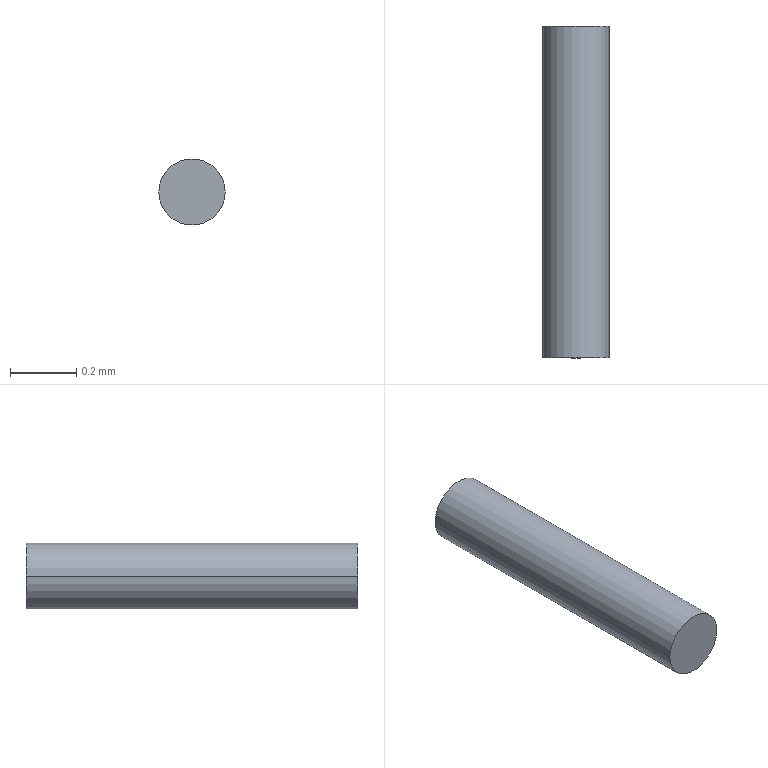Part | STEP file | Guide wheel mechanism revised.sldasm-Part-434 | 1 solid | 4 faces | box 0.2 x 1 x 0.2 mm | volume 0.03142 mm3 | cylinder 2 | plane 2 | commonest cylinder face diameters 0.2 x2
STEP:
#1=CARTESIAN_POINT('',(0.1,1.,0.));
#2=VERTEX_POINT('',#1);
#3=CARTESIAN_POINT('',(-0.1,1.,0.));
#4=VERTEX_POINT('',#3);
#5=CARTESIAN_POINT('',(0.,1.,0.));
#6=DIRECTION('',(0.,-1.,0.));
#7=DIRECTION('',(1.,0.,0.));
#8=AXIS2_PLACEMENT_3D('',#5,#6,#7);
#9=CIRCLE('',#8,0.1);
#10=EDGE_CURVE('',#2,#4,#9,.T.);
#11=ORIENTED_EDGE('',*,*,#10,.T.);
#12=CARTESIAN_POINT('',(-0.1,0.,0.));
#13=VERTEX_POINT('',#12);
#14=CARTESIAN_POINT('',(-0.1,1.,0.));
#15=DIRECTION('',(0.,-1.,0.));
#16=VECTOR('',#15,1000.);
#17=LINE('',#14,#16);
#18=EDGE_CURVE('',#4,#13,#17,.T.);
#19=ORIENTED_EDGE('',*,*,#18,.T.);
#20=CARTESIAN_POINT('',(0.1,0.,0.));
#21=VERTEX_POINT('',#20);
#22=CARTESIAN_POINT('',(0.,0.,0.));
#23=DIRECTION('',(0.,-1.,0.));
#24=DIRECTION('',(1.,0.,0.));
#25=AXIS2_PLACEMENT_3D('',#22,#23,#24);
#26=CIRCLE('',#25,0.1);
#27=EDGE_CURVE('',#21,#13,#26,.T.);
#28=ORIENTED_EDGE('',*,*,#27,.F.);
#29=CARTESIAN_POINT('',(0.1,1.,0.));
#30=DIRECTION('',(0.,-1.,0.));
#31=VECTOR('',#30,1000.);
#32=LINE('',#29,#31);
#33=EDGE_CURVE('',#2,#21,#32,.T.);
#34=ORIENTED_EDGE('',*,*,#33,.F.);
#35=EDGE_LOOP('',(#11,#19,#28,#34));
#36=FACE_OUTER_BOUND('',#35,.T.);
#37=CARTESIAN_POINT('',(0.,1.,0.));
#38=DIRECTION('',(0.,-1.,0.));
#39=DIRECTION('',(1.,0.,0.));
#40=AXIS2_PLACEMENT_3D('',#37,#38,#39);
#41=CYLINDRICAL_SURFACE('',#40,0.1);
#42=ADVANCED_FACE('',(#36),#41,.T.);
#43=ORIENTED_EDGE('',*,*,#18,.F.);
#44=CARTESIAN_POINT('',(0.,1.,0.));
#45=DIRECTION('',(0.,-1.,0.));
#46=DIRECTION('',(1.,0.,0.));
#47=AXIS2_PLACEMENT_3D('',#44,#45,#46);
#48=CIRCLE('',#47,0.1);
#49=EDGE_CURVE('',#4,#2,#48,.T.);
#50=ORIENTED_EDGE('',*,*,#49,.T.);
#51=ORIENTED_EDGE('',*,*,#33,.T.);
#52=CARTESIAN_POINT('',(0.,0.,0.));
#53=DIRECTION('',(0.,-1.,0.));
#54=DIRECTION('',(1.,0.,0.));
#55=AXIS2_PLACEMENT_3D('',#52,#53,#54);
#56=CIRCLE('',#55,0.1);
#57=EDGE_CURVE('',#13,#21,#56,.T.);
#58=ORIENTED_EDGE('',*,*,#57,.F.);
#59=EDGE_LOOP('',(#43,#50,#51,#58));
#60=FACE_OUTER_BOUND('',#59,.T.);
#61=CARTESIAN_POINT('',(0.,1.,0.));
#62=DIRECTION('',(0.,-1.,0.));
#63=DIRECTION('',(1.,0.,0.));
#64=AXIS2_PLACEMENT_3D('',#61,#62,#63);
#65=CYLINDRICAL_SURFACE('',#64,0.1);
#66=ADVANCED_FACE('',(#60),#65,.T.);
#67=ORIENTED_EDGE('',*,*,#10,.F.);
#68=ORIENTED_EDGE('',*,*,#49,.F.);
#69=EDGE_LOOP('',(#67,#68));
#70=FACE_OUTER_BOUND('',#69,.T.);
#71=CARTESIAN_POINT('',(0.,1.,0.));
#72=DIRECTION('',(0.,-1.,0.));
#73=DIRECTION('',(1.,0.,0.));
#74=AXIS2_PLACEMENT_3D('',#71,#72,#73);
#75=PLANE('',#74);
#76=ADVANCED_FACE('',(#70),#75,.F.);
#77=ORIENTED_EDGE('',*,*,#27,.T.);
#78=ORIENTED_EDGE('',*,*,#57,.T.);
#79=EDGE_LOOP('',(#77,#78));
#80=FACE_OUTER_BOUND('',#79,.T.);
#81=CARTESIAN_POINT('',(0.,0.,0.));
#82=DIRECTION('',(0.,-1.,0.));
#83=DIRECTION('',(1.,0.,0.));
#84=AXIS2_PLACEMENT_3D('',#81,#82,#83);
#85=PLANE('',#84);
#86=ADVANCED_FACE('',(#80),#85,.T.);
#87=CLOSED_SHELL('',(#42,#66,#76,#86));
#88=MANIFOLD_SOLID_BREP('',#87);
#89=CARTESIAN_POINT('',(0.,0.,0.));
#90=DIRECTION('',(0.,0.,1.));
#91=DIRECTION('',(1.,0.,0.));
#92=AXIS2_PLACEMENT_3D('',#89,#90,#91);
#93=(LENGTH_UNIT()NAMED_UNIT(*)SI_UNIT(.MILLI.,.METRE.));
#94=UNCERTAINTY_MEASURE_WITH_UNIT(LENGTH_MEASURE(0.00001),#93,'','');
#95=(NAMED_UNIT(*)PLANE_ANGLE_UNIT()SI_UNIT($,.RADIAN.));
#96=(NAMED_UNIT(*)SI_UNIT($,.STERADIAN.)SOLID_ANGLE_UNIT());
#97=(GEOMETRIC_REPRESENTATION_CONTEXT(3)GLOBAL_UNCERTAINTY_ASSIGNED_CONTEXT((#94))GLOBAL_UNIT_ASSIGNED_CONTEXT((#93,#95,#96))REPRESENTATION_CONTEXT('',''));
#98=ADVANCED_BREP_SHAPE_REPRESENTATION('',(#88,#92),#97);